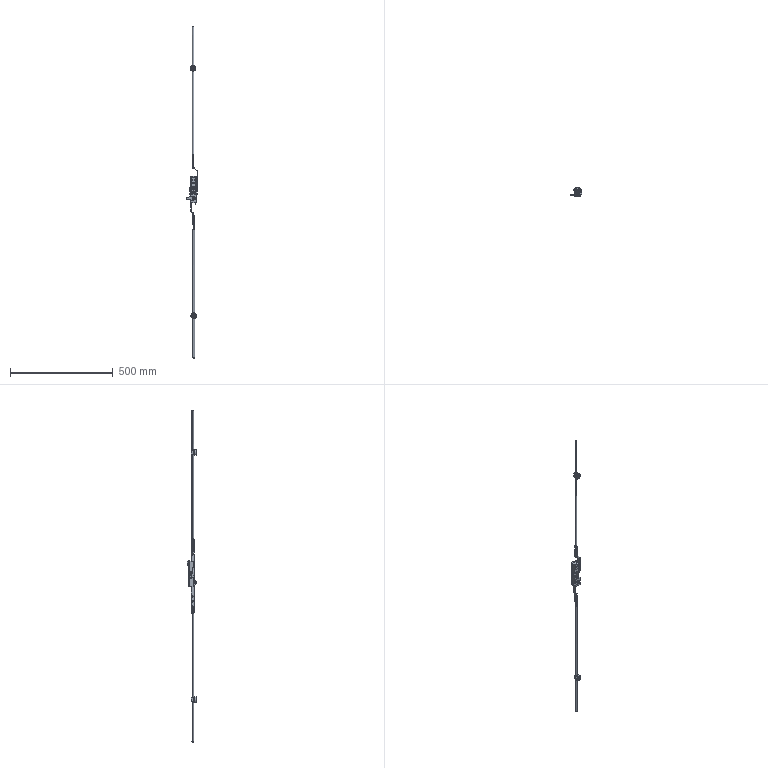Part | SolidWorks | 5 solids | 1030 faces | box 55.3 x 46.477 x 1618 mm | volume 170915 mm3 | cylinder 427 | plane 396 | spline 178 | cone 29 | commonest cylinder face diameters 1 x144 0.8 x52 6.1 x46 2 x26 16 x26 1.6 x24